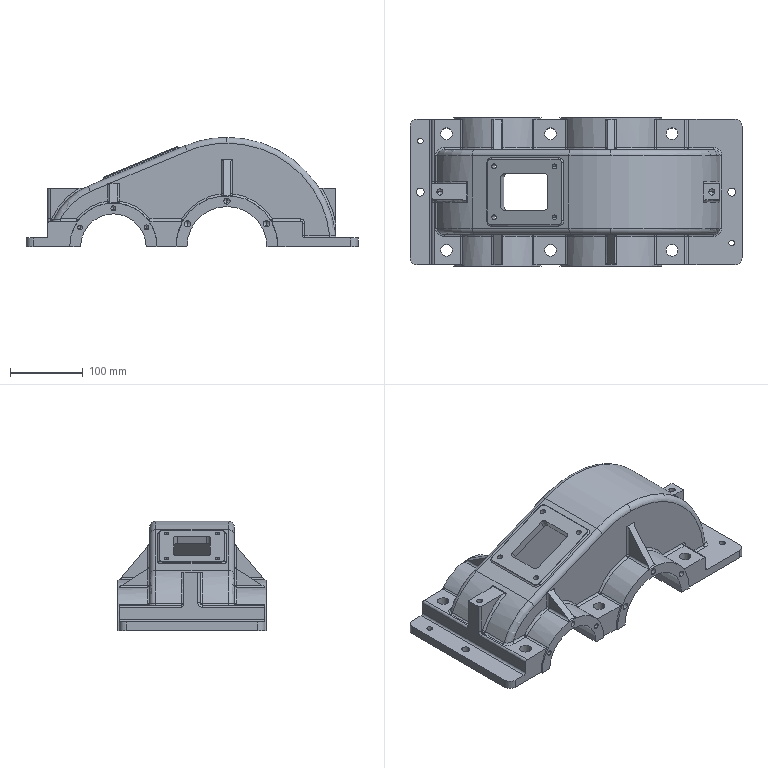Part | SolidWorks | features Fillet 21, ICE 16, 3DProfileFeature 4, HoleWzd 4, Extrusion 1, MirrorPattern 1 | 1 solid | 296 faces | box 456 x 204 x 150 mm | volume 1972353 mm3 | cylinder 143 | plane 67 | torus 32 | cone 28 | sphere 20 | spline 6 | commonest cylinder face diameters 6 x50 6.8 x20 8.5 x16 16 x14 10 x8 4 x6